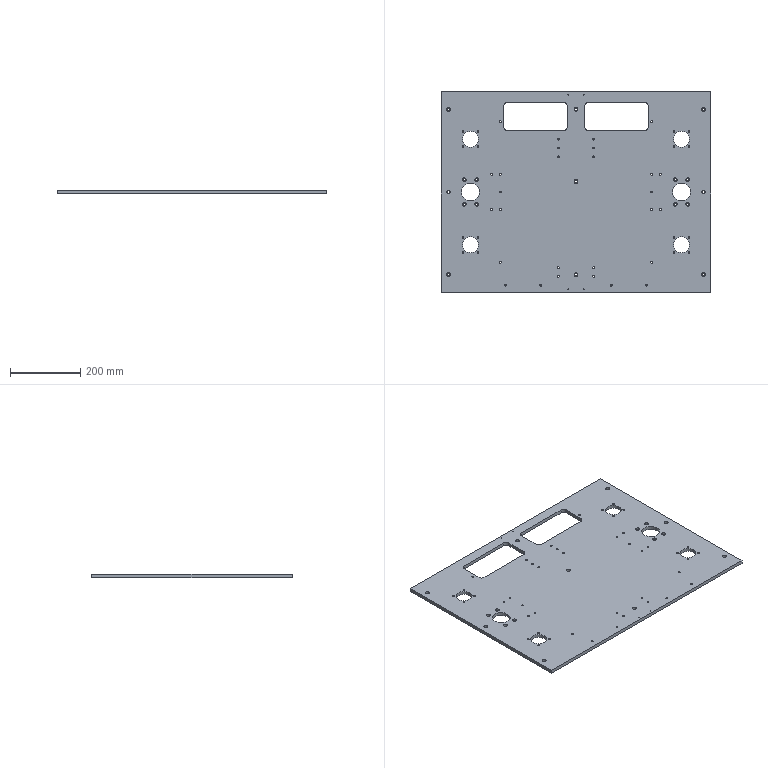Part | STEP file | Platform plate | 1 solid | 215 faces | box 765 x 570 x 10 mm | volume 3949080 mm3 | cylinder 184 | plane 31 | commonest cylinder face diameters 5 x88 6.6 x34 11 x34 2.5 x8 20 x8 45.2 x8